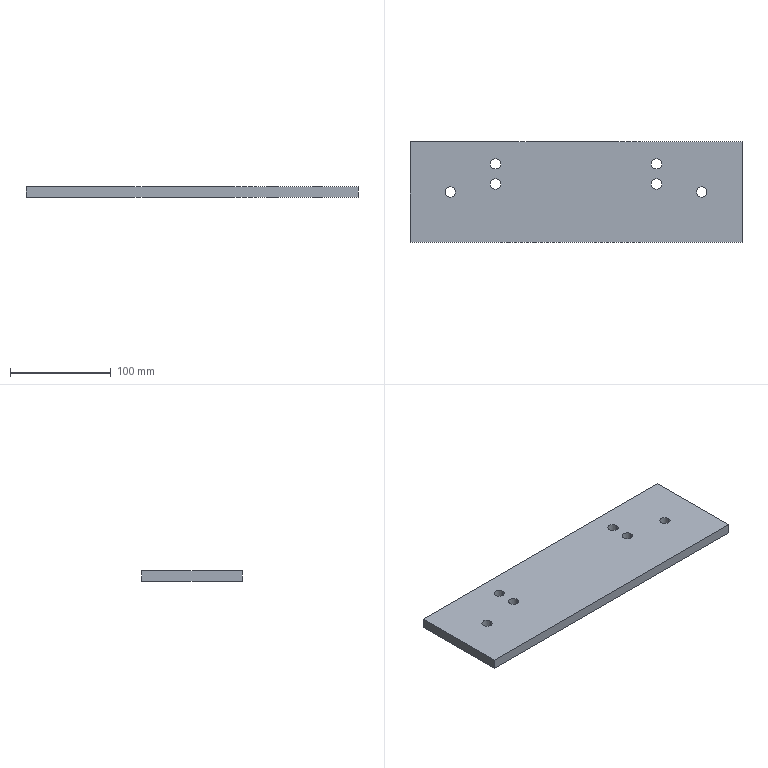Part | SolidWorks | features Extrusion 1, HoleWzd 1 | 1 solid | 18 faces | box 330 x 100 x 10 mm | volume 325097 mm3 | cylinder 12 | plane 6 | commonest cylinder face diameters 10.2 x12
STEP:
#1=CARTESIAN_POINT('',(-119.9,0.,0.));
#2=VERTEX_POINT('',#1);
#3=CARTESIAN_POINT('',(-130.1,0.,0.));
#4=VERTEX_POINT('',#3);
#5=CARTESIAN_POINT('',(-125.,0.,0.));
#6=DIRECTION('',(0.,0.,-1.));
#7=DIRECTION('',(-1.,0.,0.));
#8=AXIS2_PLACEMENT_3D('',#5,#6,#7);
#9=CIRCLE('',#8,5.1);
#10=EDGE_CURVE('',#2,#4,#9,.T.);
#11=ORIENTED_EDGE('',*,*,#10,.T.);
#12=CARTESIAN_POINT('',(-130.1,0.,10.));
#13=VERTEX_POINT('',#12);
#14=CARTESIAN_POINT('',(-130.1,0.,10.));
#15=DIRECTION('',(0.,0.,1.));
#16=VECTOR('',#15,1000.);
#17=LINE('',#14,#16);
#18=EDGE_CURVE('',#4,#13,#17,.T.);
#19=ORIENTED_EDGE('',*,*,#18,.T.);
#20=CARTESIAN_POINT('',(-119.9,0.,10.));
#21=VERTEX_POINT('',#20);
#22=CARTESIAN_POINT('',(-125.,0.,10.));
#23=DIRECTION('',(0.,0.,1.));
#24=DIRECTION('',(1.,0.,0.));
#25=AXIS2_PLACEMENT_3D('',#22,#23,#24);
#26=CIRCLE('',#25,5.1);
#27=EDGE_CURVE('',#13,#21,#26,.T.);
#28=ORIENTED_EDGE('',*,*,#27,.T.);
#29=CARTESIAN_POINT('',(-119.9,0.,10.));
#30=DIRECTION('',(0.,0.,1.));
#31=VECTOR('',#30,1000.);
#32=LINE('',#29,#31);
#33=EDGE_CURVE('',#2,#21,#32,.T.);
#34=ORIENTED_EDGE('',*,*,#33,.F.);
#35=EDGE_LOOP('',(#11,#19,#28,#34));
#36=FACE_OUTER_BOUND('',#35,.T.);
#37=CARTESIAN_POINT('',(-125.,0.,10.));
#38=DIRECTION('',(0.,0.,1.));
#39=DIRECTION('',(1.,0.,0.));
#40=AXIS2_PLACEMENT_3D('',#37,#38,#39);
#41=CYLINDRICAL_SURFACE('',#40,5.1);
#42=ADVANCED_FACE('',(#36),#41,.F.);
#43=CARTESIAN_POINT('',(-74.9,8.,0.));
#44=VERTEX_POINT('',#43);
#45=CARTESIAN_POINT('',(-85.1,8.,0.));
#46=VERTEX_POINT('',#45);
#47=CARTESIAN_POINT('',(-80.,8.,0.));
#48=DIRECTION('',(0.,0.,-1.));
#49=DIRECTION('',(-1.,0.,0.));
#50=AXIS2_PLACEMENT_3D('',#47,#48,#49);
#51=CIRCLE('',#50,5.1);
#52=EDGE_CURVE('',#44,#46,#51,.T.);
#53=ORIENTED_EDGE('',*,*,#52,.T.);
#54=CARTESIAN_POINT('',(-85.1,8.,10.));
#55=VERTEX_POINT('',#54);
#56=CARTESIAN_POINT('',(-85.1,8.,10.));
#57=DIRECTION('',(0.,0.,1.));
#58=VECTOR('',#57,1000.);
#59=LINE('',#56,#58);
#60=EDGE_CURVE('',#46,#55,#59,.T.);
#61=ORIENTED_EDGE('',*,*,#60,.T.);
#62=CARTESIAN_POINT('',(-74.9,8.,10.));
#63=VERTEX_POINT('',#62);
#64=CARTESIAN_POINT('',(-80.,8.,10.));
#65=DIRECTION('',(0.,0.,1.));
#66=DIRECTION('',(1.,0.,0.));
#67=AXIS2_PLACEMENT_3D('',#64,#65,#66);
#68=CIRCLE('',#67,5.1);
#69=EDGE_CURVE('',#55,#63,#68,.T.);
#70=ORIENTED_EDGE('',*,*,#69,.T.);
#71=CARTESIAN_POINT('',(-74.9,8.,10.));
#72=DIRECTION('',(0.,0.,1.));
#73=VECTOR('',#72,1000.);
#74=LINE('',#71,#73);
#75=EDGE_CURVE('',#44,#63,#74,.T.);
#76=ORIENTED_EDGE('',*,*,#75,.F.);
#77=EDGE_LOOP('',(#53,#61,#70,#76));
#78=FACE_OUTER_BOUND('',#77,.T.);
#79=CARTESIAN_POINT('',(-80.,8.,10.));
#80=DIRECTION('',(0.,0.,1.));
#81=DIRECTION('',(1.,0.,0.));
#82=AXIS2_PLACEMENT_3D('',#79,#80,#81);
#83=CYLINDRICAL_SURFACE('',#82,5.1);
#84=ADVANCED_FACE('',(#78),#83,.F.);
#85=CARTESIAN_POINT('',(-74.9,28.,0.));
#86=VERTEX_POINT('',#85);
#87=CARTESIAN_POINT('',(-85.1,28.,0.));
#88=VERTEX_POINT('',#87);
#89=CARTESIAN_POINT('',(-80.,28.,0.));
#90=DIRECTION('',(0.,0.,-1.));
#91=DIRECTION('',(-1.,0.,0.));
#92=AXIS2_PLACEMENT_3D('',#89,#90,#91);
#93=CIRCLE('',#92,5.1);
#94=EDGE_CURVE('',#86,#88,#93,.T.);
#95=ORIENTED_EDGE('',*,*,#94,.T.);
#96=CARTESIAN_POINT('',(-85.1,28.,10.));
#97=VERTEX_POINT('',#96);
#98=CARTESIAN_POINT('',(-85.1,28.,10.));
#99=DIRECTION('',(0.,0.,1.));
#100=VECTOR('',#99,1000.);
#101=LINE('',#98,#100);
#102=EDGE_CURVE('',#88,#97,#101,.T.);
#103=ORIENTED_EDGE('',*,*,#102,.T.);
#104=CARTESIAN_POINT('',(-74.9,28.,10.));
#105=VERTEX_POINT('',#104);
#106=CARTESIAN_POINT('',(-80.,28.,10.));
#107=DIRECTION('',(0.,0.,1.));
#108=DIRECTION('',(1.,0.,0.));
#109=AXIS2_PLACEMENT_3D('',#106,#107,#108);
#110=CIRCLE('',#109,5.1);
#111=EDGE_CURVE('',#97,#105,#110,.T.);
#112=ORIENTED_EDGE('',*,*,#111,.T.);
#113=CARTESIAN_POINT('',(-74.9,28.,10.));
#114=DIRECTION('',(0.,0.,1.));
#115=VECTOR('',#114,1000.);
#116=LINE('',#113,#115);
#117=EDGE_CURVE('',#86,#105,#116,.T.);
#118=ORIENTED_EDGE('',*,*,#117,.F.);
#119=EDGE_LOOP('',(#95,#103,#112,#118));
#120=FACE_OUTER_BOUND('',#119,.T.);
#121=CARTESIAN_POINT('',(-80.,28.,10.));
#122=DIRECTION('',(0.,0.,1.));
#123=DIRECTION('',(1.,0.,0.));
#124=AXIS2_PLACEMENT_3D('',#121,#122,#123);
#125=CYLINDRICAL_SURFACE('',#124,5.1);
#126=ADVANCED_FACE('',(#120),#125,.F.);
#127=CARTESIAN_POINT('',(85.1,28.,0.));
#128=VERTEX_POINT('',#127);
#129=CARTESIAN_POINT('',(74.9,28.,0.));
#130=VERTEX_POINT('',#129);
#131=CARTESIAN_POINT('',(80.,28.,0.));
#132=DIRECTION('',(0.,0.,-1.));
#133=DIRECTION('',(-1.,0.,0.));
#134=AXIS2_PLACEMENT_3D('',#131,#132,#133);
#135=CIRCLE('',#134,5.1);
#136=EDGE_CURVE('',#128,#130,#135,.T.);
#137=ORIENTED_EDGE('',*,*,#136,.T.);
#138=CARTESIAN_POINT('',(74.9,28.,10.));
#139=VERTEX_POINT('',#138);
#140=CARTESIAN_POINT('',(74.9,28.,10.));
#141=DIRECTION('',(0.,0.,1.));
#142=VECTOR('',#141,1000.);
#143=LINE('',#140,#142);
#144=EDGE_CURVE('',#130,#139,#143,.T.);
#145=ORIENTED_EDGE('',*,*,#144,.T.);
#146=CARTESIAN_POINT('',(85.1,28.,10.));
#147=VERTEX_POINT('',#146);
#148=CARTESIAN_POINT('',(80.,28.,10.));
#149=DIRECTION('',(0.,0.,1.));
#150=DIRECTION('',(1.,0.,0.));
#151=AXIS2_PLACEMENT_3D('',#148,#149,#150);
#152=CIRCLE('',#151,5.1);
#153=EDGE_CURVE('',#139,#147,#152,.T.);
#154=ORIENTED_EDGE('',*,*,#153,.T.);
#155=CARTESIAN_POINT('',(85.1,28.,10.));
#156=DIRECTION('',(0.,0.,1.));
#157=VECTOR('',#156,1000.);
#158=LINE('',#155,#157);
#159=EDGE_CURVE('',#128,#147,#158,.T.);
#160=ORIENTED_EDGE('',*,*,#159,.F.);
#161=EDGE_LOOP('',(#137,#145,#154,#160));
#162=FACE_OUTER_BOUND('',#161,.T.);
#163=CARTESIAN_POINT('',(80.,28.,10.));
#164=DIRECTION('',(0.,0.,1.));
#165=DIRECTION('',(1.,0.,0.));
#166=AXIS2_PLACEMENT_3D('',#163,#164,#165);
#167=CYLINDRICAL_SURFACE('',#166,5.1);
#168=ADVANCED_FACE('',(#162),#167,.F.);
#169=CARTESIAN_POINT('',(85.1,8.,0.));
#170=VERTEX_POINT('',#169);
#171=CARTESIAN_POINT('',(74.9,8.,0.));
#172=VERTEX_POINT('',#171);
#173=CARTESIAN_POINT('',(80.,8.,0.));
#174=DIRECTION('',(0.,0.,-1.));
#175=DIRECTION('',(-1.,0.,0.));
#176=AXIS2_PLACEMENT_3D('',#173,#174,#175);
#177=CIRCLE('',#176,5.1);
#178=EDGE_CURVE('',#170,#172,#177,.T.);
#179=ORIENTED_EDGE('',*,*,#178,.T.);
#180=CARTESIAN_POINT('',(74.9,8.,10.));
#181=VERTEX_POINT('',#180);
#182=CARTESIAN_POINT('',(74.9,8.,10.));
#183=DIRECTION('',(0.,0.,1.));
#184=VECTOR('',#183,1000.);
#185=LINE('',#182,#184);
#186=EDGE_CURVE('',#172,#181,#185,.T.);
#187=ORIENTED_EDGE('',*,*,#186,.T.);
#188=CARTESIAN_POINT('',(85.1,8.,10.));
#189=VERTEX_POINT('',#188);
#190=CARTESIAN_POINT('',(80.,8.,10.));
#191=DIRECTION('',(0.,0.,1.));
#192=DIRECTION('',(1.,0.,0.));
#193=AXIS2_PLACEMENT_3D('',#190,#191,#192);
#194=CIRCLE('',#193,5.1);
#195=EDGE_CURVE('',#181,#189,#194,.T.);
#196=ORIENTED_EDGE('',*,*,#195,.T.);
#197=CARTESIAN_POINT('',(85.1,8.,10.));
#198=DIRECTION('',(0.,0.,1.));
#199=VECTOR('',#198,1000.);
#200=LINE('',#197,#199);
#201=EDGE_CURVE('',#170,#189,#200,.T.);
#202=ORIENTED_EDGE('',*,*,#201,.F.);
#203=EDGE_LOOP('',(#179,#187,#196,#202));
#204=FACE_OUTER_BOUND('',#203,.T.);
#205=CARTESIAN_POINT('',(80.,8.,10.));
#206=DIRECTION('',(0.,0.,1.));
#207=DIRECTION('',(1.,0.,0.));
#208=AXIS2_PLACEMENT_3D('',#205,#206,#207);
#209=CYLINDRICAL_SURFACE('',#208,5.1);
#210=ADVANCED_FACE('',(#204),#209,.F.);
#211=CARTESIAN_POINT('',(130.1,0.,0.));
#212=VERTEX_POINT('',#211);
#213=CARTESIAN_POINT('',(119.9,0.,0.));
#214=VERTEX_POINT('',#213);
#215=CARTESIAN_POINT('',(125.,0.,0.));
#216=DIRECTION('',(0.,0.,-1.));
#217=DIRECTION('',(-1.,0.,0.));
#218=AXIS2_PLACEMENT_3D('',#215,#216,#217);
#219=CIRCLE('',#218,5.1);
#220=EDGE_CURVE('',#212,#214,#219,.T.);
#221=ORIENTED_EDGE('',*,*,#220,.T.);
#222=CARTESIAN_POINT('',(119.9,0.,10.));
#223=VERTEX_POINT('',#222);
#224=CARTESIAN_POINT('',(119.9,0.,10.));
#225=DIRECTION('',(0.,0.,1.));
#226=VECTOR('',#225,1000.);
#227=LINE('',#224,#226);
#228=EDGE_CURVE('',#214,#223,#227,.T.);
#229=ORIENTED_EDGE('',*,*,#228,.T.);
#230=CARTESIAN_POINT('',(130.1,0.,10.));
#231=VERTEX_POINT('',#230);
#232=CARTESIAN_POINT('',(125.,0.,10.));
#233=DIRECTION('',(0.,0.,1.));
#234=DIRECTION('',(1.,0.,0.));
#235=AXIS2_PLACEMENT_3D('',#232,#233,#234);
#236=CIRCLE('',#235,5.1);
#237=EDGE_CURVE('',#223,#231,#236,.T.);
#238=ORIENTED_EDGE('',*,*,#237,.T.);
#239=CARTESIAN_POINT('',(130.1,0.,10.));
#240=DIRECTION('',(0.,0.,1.));
#241=VECTOR('',#240,1000.);
#242=LINE('',#239,#241);
#243=EDGE_CURVE('',#212,#231,#242,.T.);
#244=ORIENTED_EDGE('',*,*,#243,.F.);
#245=EDGE_LOOP('',(#221,#229,#238,#244));
#246=FACE_OUTER_BOUND('',#245,.T.);
#247=CARTESIAN_POINT('',(125.,0.,10.));
#248=DIRECTION('',(0.,0.,1.));
#249=DIRECTION('',(1.,0.,0.));
#250=AXIS2_PLACEMENT_3D('',#247,#248,#249);
#251=CYLINDRICAL_SURFACE('',#250,5.1);
#252=ADVANCED_FACE('',(#246),#251,.F.);
#253=CARTESIAN_POINT('',(-165.,-50.,0.));
#254=VERTEX_POINT('',#253);
#255=CARTESIAN_POINT('',(165.,-50.,0.));
#256=VERTEX_POINT('',#255);
#257=CARTESIAN_POINT('',(-165.,-50.,0.));
#258=DIRECTION('',(1.,0.,0.));
#259=VECTOR('',#258,1000.);
#260=LINE('',#257,#259);
#261=EDGE_CURVE('',#254,#256,#260,.T.);
#262=ORIENTED_EDGE('',*,*,#261,.T.);
#263=CARTESIAN_POINT('',(165.,-50.,10.));
#264=VERTEX_POINT('',#263);
#265=CARTESIAN_POINT('',(165.,-50.,10.));
#266=DIRECTION('',(0.,0.,-1.));
#267=VECTOR('',#266,1000.);
#268=LINE('',#265,#267);
#269=EDGE_CURVE('',#264,#256,#268,.T.);
#270=ORIENTED_EDGE('',*,*,#269,.F.);
#271=CARTESIAN_POINT('',(-165.,-50.,10.));
#272=VERTEX_POINT('',#271);
#273=CARTESIAN_POINT('',(-165.,-50.,10.));
#274=DIRECTION('',(1.,0.,0.));
#275=VECTOR('',#274,1000.);
#276=LINE('',#273,#275);
#277=EDGE_CURVE('',#272,#264,#276,.T.);
#278=ORIENTED_EDGE('',*,*,#277,.F.);
#279=CARTESIAN_POINT('',(-165.,-50.,10.));
#280=DIRECTION('',(0.,0.,-1.));
#281=VECTOR('',#280,1000.);
#282=LINE('',#279,#281);
#283=EDGE_CURVE('',#272,#254,#282,.T.);
#284=ORIENTED_EDGE('',*,*,#283,.T.);
#285=EDGE_LOOP('',(#262,#270,#278,#284));
#286=FACE_OUTER_BOUND('',#285,.T.);
#287=CARTESIAN_POINT('',(-165.,-50.,10.));
#288=DIRECTION('',(0.,1.,0.));
#289=DIRECTION('',(0.,0.,1.));
#290=AXIS2_PLACEMENT_3D('',#287,#288,#289);
#291=PLANE('',#290);
#292=ADVANCED_FACE('',(#286),#291,.F.);
#293=CARTESIAN_POINT('',(165.,50.,0.));
#294=VERTEX_POINT('',#293);
#295=CARTESIAN_POINT('',(165.,50.,0.));
#296=DIRECTION('',(0.,-1.,0.));
#297=VECTOR('',#296,1000.);
#298=LINE('',#295,#297);
#299=EDGE_CURVE('',#294,#256,#298,.T.);
#300=ORIENTED_EDGE('',*,*,#299,.F.);
#301=CARTESIAN_POINT('',(165.,50.,10.));
#302=VERTEX_POINT('',#301);
#303=CARTESIAN_POINT('',(165.,50.,10.));
#304=DIRECTION('',(0.,0.,-1.));
#305=VECTOR('',#304,1000.);
#306=LINE('',#303,#305);
#307=EDGE_CURVE('',#302,#294,#306,.T.);
#308=ORIENTED_EDGE('',*,*,#307,.F.);
#309=CARTESIAN_POINT('',(165.,50.,10.));
#310=DIRECTION('',(0.,-1.,0.));
#311=VECTOR('',#310,1000.);
#312=LINE('',#309,#311);
#313=EDGE_CURVE('',#302,#264,#312,.T.);
#314=ORIENTED_EDGE('',*,*,#313,.T.);
#315=ORIENTED_EDGE('',*,*,#269,.T.);
#316=EDGE_LOOP('',(#300,#308,#314,#315));
#317=FACE_OUTER_BOUND('',#316,.T.);
#318=CARTESIAN_POINT('',(165.,50.,10.));
#319=DIRECTION('',(1.,0.,0.));
#320=DIRECTION('',(0.,1.,0.));
#321=AXIS2_PLACEMENT_3D('',#318,#319,#320);
#322=PLANE('',#321);
#323=ADVANCED_FACE('',(#317),#322,.T.);
#324=CARTESIAN_POINT('',(-165.,50.,0.));
#325=VERTEX_POINT('',#324);
#326=CARTESIAN_POINT('',(-165.,50.,0.));
#327=DIRECTION('',(1.,0.,0.));
#328=VECTOR('',#327,1000.);
#329=LINE('',#326,#328);
#330=EDGE_CURVE('',#325,#294,#329,.T.);
#331=ORIENTED_EDGE('',*,*,#330,.F.);
#332=CARTESIAN_POINT('',(-165.,50.,10.));
#333=VERTEX_POINT('',#332);
#334=CARTESIAN_POINT('',(-165.,50.,10.));
#335=DIRECTION('',(0.,0.,-1.));
#336=VECTOR('',#335,1000.);
#337=LINE('',#334,#336);
#338=EDGE_CURVE('',#333,#325,#337,.T.);
#339=ORIENTED_EDGE('',*,*,#338,.F.);
#340=CARTESIAN_POINT('',(-165.,50.,10.));
#341=DIRECTION('',(1.,0.,0.));
#342=VECTOR('',#341,1000.);
#343=LINE('',#340,#342);
#344=EDGE_CURVE('',#333,#302,#343,.T.);
#345=ORIENTED_EDGE('',*,*,#344,.T.);
#346=ORIENTED_EDGE('',*,*,#307,.T.);
#347=EDGE_LOOP('',(#331,#339,#345,#346));
#348=FACE_OUTER_BOUND('',#347,.T.);
#349=CARTESIAN_POINT('',(-165.,50.,10.));
#350=DIRECTION('',(0.,1.,0.));
#351=DIRECTION('',(0.,0.,1.));
#352=AXIS2_PLACEMENT_3D('',#349,#350,#351);
#353=PLANE('',#352);
#354=ADVANCED_FACE('',(#348),#353,.T.);
#355=CARTESIAN_POINT('',(-165.,50.,0.));
#356=DIRECTION('',(0.,-1.,0.));
#357=VECTOR('',#356,1000.);
#358=LINE('',#355,#357);
#359=EDGE_CURVE('',#325,#254,#358,.T.);
#360=ORIENTED_EDGE('',*,*,#359,.T.);
#361=ORIENTED_EDGE('',*,*,#283,.F.);
#362=CARTESIAN_POINT('',(-165.,50.,10.));
#363=DIRECTION('',(0.,-1.,0.));
#364=VECTOR('',#363,1000.);
#365=LINE('',#362,#364);
#366=EDGE_CURVE('',#333,#272,#365,.T.);
#367=ORIENTED_EDGE('',*,*,#366,.F.);
#368=ORIENTED_EDGE('',*,*,#338,.T.);
#369=EDGE_LOOP('',(#360,#361,#367,#368));
#370=FACE_OUTER_BOUND('',#369,.T.);
#371=CARTESIAN_POINT('',(-165.,50.,10.));
#372=DIRECTION('',(1.,0.,0.));
#373=DIRECTION('',(0.,1.,0.));
#374=AXIS2_PLACEMENT_3D('',#371,#372,#373);
#375=PLANE('',#374);
#376=ADVANCED_FACE('',(#370),#375,.F.);
#377=CARTESIAN_POINT('',(-125.,0.,10.));
#378=DIRECTION('',(0.,0.,1.));
#379=DIRECTION('',(1.,0.,0.));
#380=AXIS2_PLACEMENT_3D('',#377,#378,#379);
#381=CIRCLE('',#380,5.1);
#382=EDGE_CURVE('',#21,#13,#381,.T.);
#383=ORIENTED_EDGE('',*,*,#382,.F.);
#384=ORIENTED_EDGE('',*,*,#27,.F.);
#385=EDGE_LOOP('',(#383,#384));
#386=FACE_BOUND('',#385,.T.);
#387=CARTESIAN_POINT('',(-80.,8.,10.));
#388=DIRECTION('',(0.,0.,1.));
#389=DIRECTION('',(1.,0.,0.));
#390=AXIS2_PLACEMENT_3D('',#387,#388,#389);
#391=CIRCLE('',#390,5.1);
#392=EDGE_CURVE('',#63,#55,#391,.T.);
#393=ORIENTED_EDGE('',*,*,#392,.F.);
#394=ORIENTED_EDGE('',*,*,#69,.F.);
#395=EDGE_LOOP('',(#393,#394));
#396=FACE_BOUND('',#395,.T.);
#397=CARTESIAN_POINT('',(-80.,28.,10.));
#398=DIRECTION('',(0.,0.,1.));
#399=DIRECTION('',(1.,0.,0.));
#400=AXIS2_PLACEMENT_3D('',#397,#398,#399);
#401=CIRCLE('',#400,5.1);
#402=EDGE_CURVE('',#105,#97,#401,.T.);
#403=ORIENTED_EDGE('',*,*,#402,.F.);
#404=ORIENTED_EDGE('',*,*,#111,.F.);
#405=EDGE_LOOP('',(#403,#404));
#406=FACE_BOUND('',#405,.T.);
#407=CARTESIAN_POINT('',(80.,28.,10.));
#408=DIRECTION('',(0.,0.,1.));
#409=DIRECTION('',(1.,0.,0.));
#410=AXIS2_PLACEMENT_3D('',#407,#408,#409);
#411=CIRCLE('',#410,5.1);
#412=EDGE_CURVE('',#147,#139,#411,.T.);
#413=ORIENTED_EDGE('',*,*,#412,.F.);
#414=ORIENTED_EDGE('',*,*,#153,.F.);
#415=EDGE_LOOP('',(#413,#414));
#416=FACE_BOUND('',#415,.T.);
#417=CARTESIAN_POINT('',(80.,8.,10.));
#418=DIRECTION('',(0.,0.,1.));
#419=DIRECTION('',(1.,0.,0.));
#420=AXIS2_PLACEMENT_3D('',#417,#418,#419);
#421=CIRCLE('',#420,5.1);
#422=EDGE_CURVE('',#189,#181,#421,.T.);
#423=ORIENTED_EDGE('',*,*,#422,.F.);
#424=ORIENTED_EDGE('',*,*,#195,.F.);
#425=EDGE_LOOP('',(#423,#424));
#426=FACE_BOUND('',#425,.T.);
#427=CARTESIAN_POINT('',(125.,0.,10.));
#428=DIRECTION('',(0.,0.,1.));
#429=DIRECTION('',(1.,0.,0.));
#430=AXIS2_PLACEMENT_3D('',#427,#428,#429);
#431=CIRCLE('',#430,5.1);
#432=EDGE_CURVE('',#231,#223,#431,.T.);
#433=ORIENTED_EDGE('',*,*,#432,.F.);
#434=ORIENTED_EDGE('',*,*,#237,.F.);
#435=EDGE_LOOP('',(#433,#434));
#436=FACE_BOUND('',#435,.T.);
#437=ORIENTED_EDGE('',*,*,#277,.T.);
#438=ORIENTED_EDGE('',*,*,#313,.F.);
#439=ORIENTED_EDGE('',*,*,#344,.F.);
#440=ORIENTED_EDGE('',*,*,#366,.T.);
#441=EDGE_LOOP('',(#437,#438,#439,#440));
#442=FACE_OUTER_BOUND('',#441,.T.);
#443=CARTESIAN_POINT('',(0.,0.,10.));
#444=DIRECTION('',(0.,0.,-1.));
#445=DIRECTION('',(-1.,0.,0.));
#446=AXIS2_PLACEMENT_3D('',#443,#444,#445);
#447=PLANE('',#446);
#448=ADVANCED_FACE('',(#386,#396,#406,#416,#426,#436,#442),#447,.F.);
#449=ORIENTED_EDGE('',*,*,#10,.F.);
#450=CARTESIAN_POINT('',(-125.,0.,0.));
#451=DIRECTION('',(0.,0.,-1.));
#452=DIRECTION('',(-1.,0.,0.));
#453=AXIS2_PLACEMENT_3D('',#450,#451,#452);
#454=CIRCLE('',#453,5.1);
#455=EDGE_CURVE('',#4,#2,#454,.T.);
#456=ORIENTED_EDGE('',*,*,#455,.F.);
#457=EDGE_LOOP('',(#449,#456));
#458=FACE_BOUND('',#457,.T.);
#459=ORIENTED_EDGE('',*,*,#52,.F.);
#460=CARTESIAN_POINT('',(-80.,8.,0.));
#461=DIRECTION('',(0.,0.,-1.));
#462=DIRECTION('',(-1.,0.,0.));
#463=AXIS2_PLACEMENT_3D('',#460,#461,#462);
#464=CIRCLE('',#463,5.1);
#465=EDGE_CURVE('',#46,#44,#464,.T.);
#466=ORIENTED_EDGE('',*,*,#465,.F.);
#467=EDGE_LOOP('',(#459,#466));
#468=FACE_BOUND('',#467,.T.);
#469=ORIENTED_EDGE('',*,*,#94,.F.);
#470=CARTESIAN_POINT('',(-80.,28.,0.));
#471=DIRECTION('',(0.,0.,-1.));
#472=DIRECTION('',(-1.,0.,0.));
#473=AXIS2_PLACEMENT_3D('',#470,#471,#472);
#474=CIRCLE('',#473,5.1);
#475=EDGE_CURVE('',#88,#86,#474,.T.);
#476=ORIENTED_EDGE('',*,*,#475,.F.);
#477=EDGE_LOOP('',(#469,#476));
#478=FACE_BOUND('',#477,.T.);
#479=ORIENTED_EDGE('',*,*,#136,.F.);
#480=CARTESIAN_POINT('',(80.,28.,0.));
#481=DIRECTION('',(0.,0.,-1.));
#482=DIRECTION('',(-1.,0.,0.));
#483=AXIS2_PLACEMENT_3D('',#480,#481,#482);
#484=CIRCLE('',#483,5.1);
#485=EDGE_CURVE('',#130,#128,#484,.T.);
#486=ORIENTED_EDGE('',*,*,#485,.F.);
#487=EDGE_LOOP('',(#479,#486));
#488=FACE_BOUND('',#487,.T.);
#489=ORIENTED_EDGE('',*,*,#178,.F.);
#490=CARTESIAN_POINT('',(80.,8.,0.));
#491=DIRECTION('',(0.,0.,-1.));
#492=DIRECTION('',(-1.,0.,0.));
#493=AXIS2_PLACEMENT_3D('',#490,#491,#492);
#494=CIRCLE('',#493,5.1);
#495=EDGE_CURVE('',#172,#170,#494,.T.);
#496=ORIENTED_EDGE('',*,*,#495,.F.);
#497=EDGE_LOOP('',(#489,#496));
#498=FACE_BOUND('',#497,.T.);
#499=ORIENTED_EDGE('',*,*,#220,.F.);
#500=CARTESIAN_POINT('',(125.,0.,0.));
#501=DIRECTION('',(0.,0.,-1.));
#502=DIRECTION('',(-1.,0.,0.));
#503=AXIS2_PLACEMENT_3D('',#500,#501,#502);
#504=CIRCLE('',#503,5.1);
#505=EDGE_CURVE('',#214,#212,#504,.T.);
#506=ORIENTED_EDGE('',*,*,#505,.F.);
#507=EDGE_LOOP('',(#499,#506));
#508=FACE_BOUND('',#507,.T.);
#509=ORIENTED_EDGE('',*,*,#261,.F.);
#510=ORIENTED_EDGE('',*,*,#359,.F.);
#511=ORIENTED_EDGE('',*,*,#330,.T.);
#512=ORIENTED_EDGE('',*,*,#299,.T.);
#513=EDGE_LOOP('',(#509,#510,#511,#512));
#514=FACE_OUTER_BOUND('',#513,.T.);
#515=CARTESIAN_POINT('',(0.,0.,0.));
#516=DIRECTION('',(0.,0.,-1.));
#517=DIRECTION('',(-1.,0.,0.));
#518=AXIS2_PLACEMENT_3D('',#515,#516,#517);
#519=PLANE('',#518);
#520=ADVANCED_FACE('',(#458,#468,#478,#488,#498,#508,#514),#519,.T.);
#521=ORIENTED_EDGE('',*,*,#228,.F.);
#522=ORIENTED_EDGE('',*,*,#505,.T.);
#523=ORIENTED_EDGE('',*,*,#243,.T.);
#524=ORIENTED_EDGE('',*,*,#432,.T.);
#525=EDGE_LOOP('',(#521,#522,#523,#524));
#526=FACE_OUTER_BOUND('',#525,.T.);
#527=CARTESIAN_POINT('',(125.,0.,10.));
#528=DIRECTION('',(0.,0.,1.));
#529=DIRECTION('',(1.,0.,0.));
#530=AXIS2_PLACEMENT_3D('',#527,#528,#529);
#531=CYLINDRICAL_SURFACE('',#530,5.1);
#532=ADVANCED_FACE('',(#526),#531,.F.);
#533=ORIENTED_EDGE('',*,*,#186,.F.);
#534=ORIENTED_EDGE('',*,*,#495,.T.);
#535=ORIENTED_EDGE('',*,*,#201,.T.);
#536=ORIENTED_EDGE('',*,*,#422,.T.);
#537=EDGE_LOOP('',(#533,#534,#535,#536));
#538=FACE_OUTER_BOUND('',#537,.T.);
#539=CARTESIAN_POINT('',(80.,8.,10.));
#540=DIRECTION('',(0.,0.,1.));
#541=DIRECTION('',(1.,0.,0.));
#542=AXIS2_PLACEMENT_3D('',#539,#540,#541);
#543=CYLINDRICAL_SURFACE('',#542,5.1);
#544=ADVANCED_FACE('',(#538),#543,.F.);
#545=ORIENTED_EDGE('',*,*,#144,.F.);
#546=ORIENTED_EDGE('',*,*,#485,.T.);
#547=ORIENTED_EDGE('',*,*,#159,.T.);
#548=ORIENTED_EDGE('',*,*,#412,.T.);
#549=EDGE_LOOP('',(#545,#546,#547,#548));
#550=FACE_OUTER_BOUND('',#549,.T.);
#551=CARTESIAN_POINT('',(80.,28.,10.));
#552=DIRECTION('',(0.,0.,1.));
#553=DIRECTION('',(1.,0.,0.));
#554=AXIS2_PLACEMENT_3D('',#551,#552,#553);
#555=CYLINDRICAL_SURFACE('',#554,5.1);
#556=ADVANCED_FACE('',(#550),#555,.F.);
#557=ORIENTED_EDGE('',*,*,#102,.F.);
#558=ORIENTED_EDGE('',*,*,#475,.T.);
#559=ORIENTED_EDGE('',*,*,#117,.T.);
#560=ORIENTED_EDGE('',*,*,#402,.T.);
#561=EDGE_LOOP('',(#557,#558,#559,#560));
#562=FACE_OUTER_BOUND('',#561,.T.);
#563=CARTESIAN_POINT('',(-80.,28.,10.));
#564=DIRECTION('',(0.,0.,1.));
#565=DIRECTION('',(1.,0.,0.));
#566=AXIS2_PLACEMENT_3D('',#563,#564,#565);
#567=CYLINDRICAL_SURFACE('',#566,5.1);
#568=ADVANCED_FACE('',(#562),#567,.F.);
#569=ORIENTED_EDGE('',*,*,#60,.F.);
#570=ORIENTED_EDGE('',*,*,#465,.T.);
#571=ORIENTED_EDGE('',*,*,#75,.T.);
#572=ORIENTED_EDGE('',*,*,#392,.T.);
#573=EDGE_LOOP('',(#569,#570,#571,#572));
#574=FACE_OUTER_BOUND('',#573,.T.);
#575=CARTESIAN_POINT('',(-80.,8.,10.));
#576=DIRECTION('',(0.,0.,1.));
#577=DIRECTION('',(1.,0.,0.));
#578=AXIS2_PLACEMENT_3D('',#575,#576,#577);
#579=CYLINDRICAL_SURFACE('',#578,5.1);
#580=ADVANCED_FACE('',(#574),#579,.F.);
#581=ORIENTED_EDGE('',*,*,#18,.F.);
#582=ORIENTED_EDGE('',*,*,#455,.T.);
#583=ORIENTED_EDGE('',*,*,#33,.T.);
#584=ORIENTED_EDGE('',*,*,#382,.T.);
#585=EDGE_LOOP('',(#581,#582,#583,#584));
#586=FACE_OUTER_BOUND('',#585,.T.);
#587=CARTESIAN_POINT('',(-125.,0.,10.));
#588=DIRECTION('',(0.,0.,1.));
#589=DIRECTION('',(1.,0.,0.));
#590=AXIS2_PLACEMENT_3D('',#587,#588,#589);
#591=CYLINDRICAL_SURFACE('',#590,5.1);
#592=ADVANCED_FACE('',(#586),#591,.F.);
#593=CLOSED_SHELL('',(#42,#84,#126,#168,#210,#252,#292,#323,#354,#376,#448,#520,#532,#544,#556,#568,#580,#592));
#594=MANIFOLD_SOLID_BREP('',#593);
#595=CARTESIAN_POINT('',(0.,0.,0.));
#596=DIRECTION('',(0.,0.,1.));
#597=DIRECTION('',(1.,0.,0.));
#598=AXIS2_PLACEMENT_3D('',#595,#596,#597);
#599=(LENGTH_UNIT()NAMED_UNIT(*)SI_UNIT(.MILLI.,.METRE.));
#600=UNCERTAINTY_MEASURE_WITH_UNIT(LENGTH_MEASURE(0.00001),#599,'','');
#601=(NAMED_UNIT(*)PLANE_ANGLE_UNIT()SI_UNIT($,.RADIAN.));
#602=(NAMED_UNIT(*)SI_UNIT($,.STERADIAN.)SOLID_ANGLE_UNIT());
#603=(GEOMETRIC_REPRESENTATION_CONTEXT(3)GLOBAL_UNCERTAINTY_ASSIGNED_CONTEXT((#600))GLOBAL_UNIT_ASSIGNED_CONTEXT((#599,#601,#602))REPRESENTATION_CONTEXT('',''));
#604=ADVANCED_BREP_SHAPE_REPRESENTATION('',(#594,#598),#603);